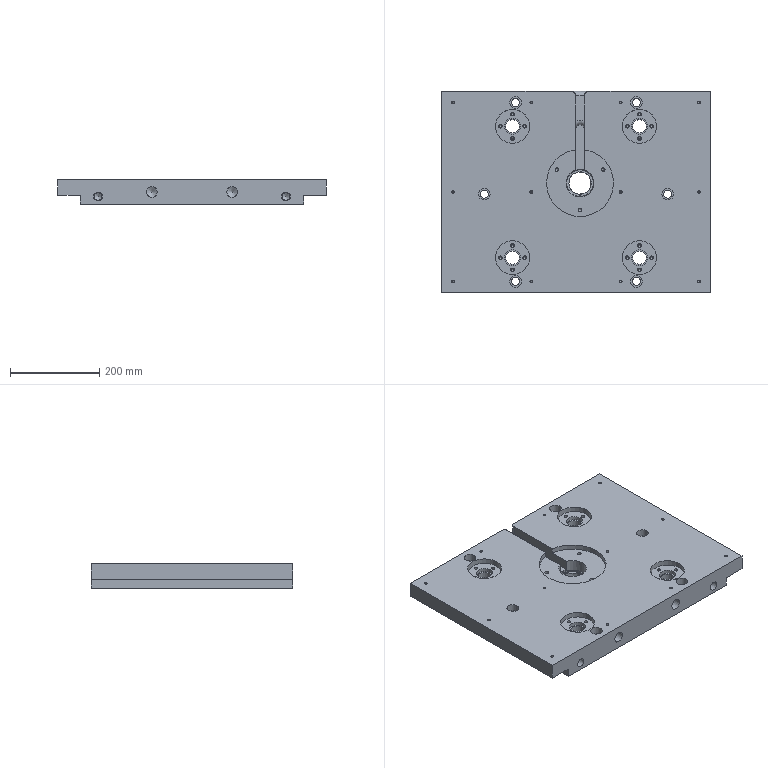Part | STEP file | AD | 1 solid | 213 faces | box 600 x 450 x 55 mm | volume 12937855 mm3 | cylinder 102 | plane 71 | cone 39 | torus 1 | commonest cylinder face diameters 6.7 x19 8 x19 5 x12 6 x12 18 x6 20 x6